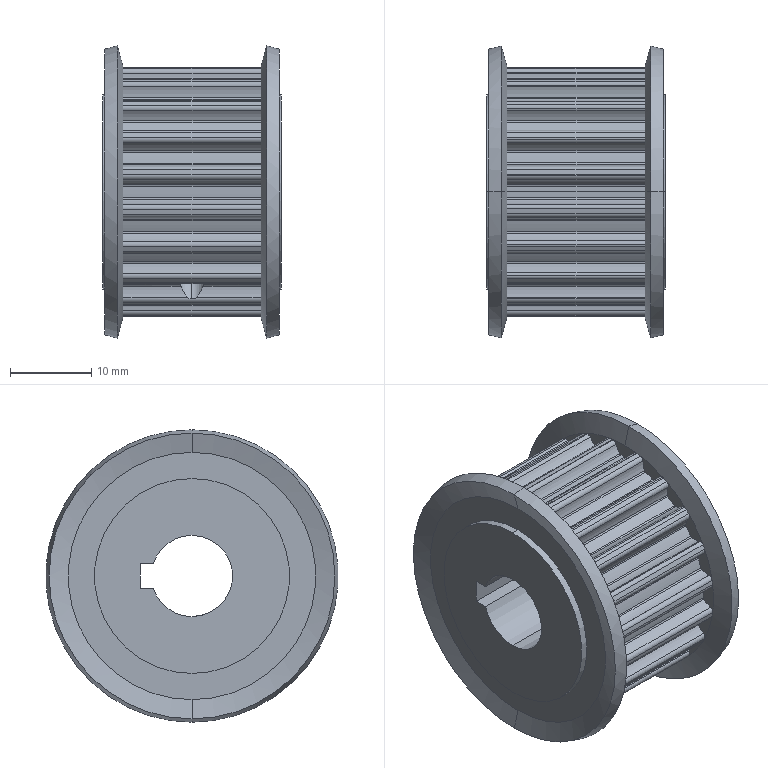Part | SolidWorks | features BaseBody 1 | 1 solid | 265 faces | box 22 x 36 x 36 mm | volume 13176 mm3 | cylinder 203 | plane 50 | cone 12 | commonest cylinder face diameters 0.5 x51 1.1 x50 6.55 x48 27.33 x23 30.87 x20 3.242 x4